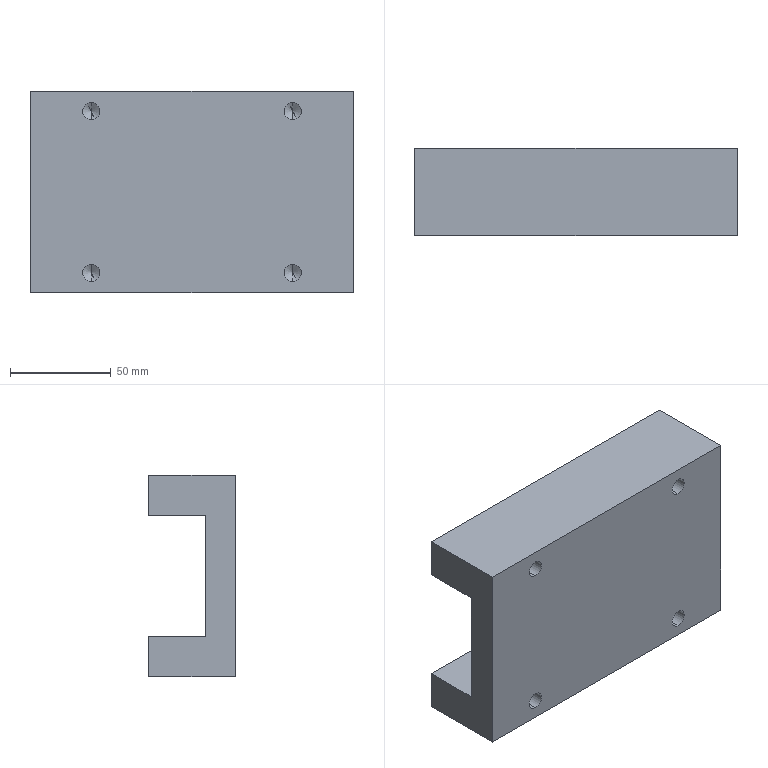Part | STEP file | 1 solid | 42 faces | box 160 x 43 x 100 mm | volume 410478 mm3 | cylinder 16 | cone 16 | plane 10 | commonest cylinder face diameters 6.8 x8 8.5 x8